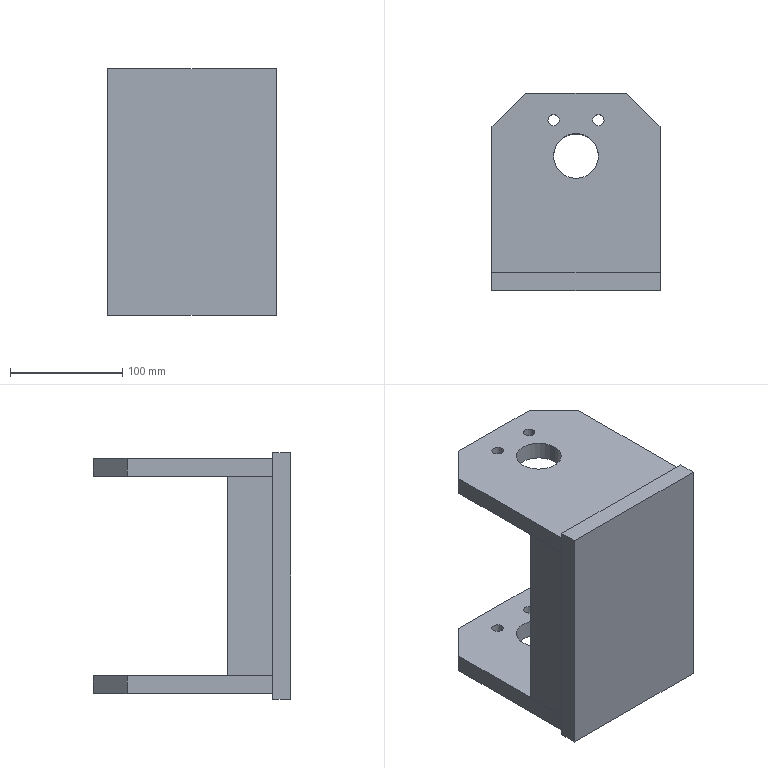Part | STEP file | Hanging sprocket seat | 5 solids | 54 faces | box 150 x 176 x 220 mm | volume 1392367 mm3 | plane 34 | cylinder 16 | cone 4 | commonest cylinder face diameters 10.2 x8 3.3 x4 40 x4